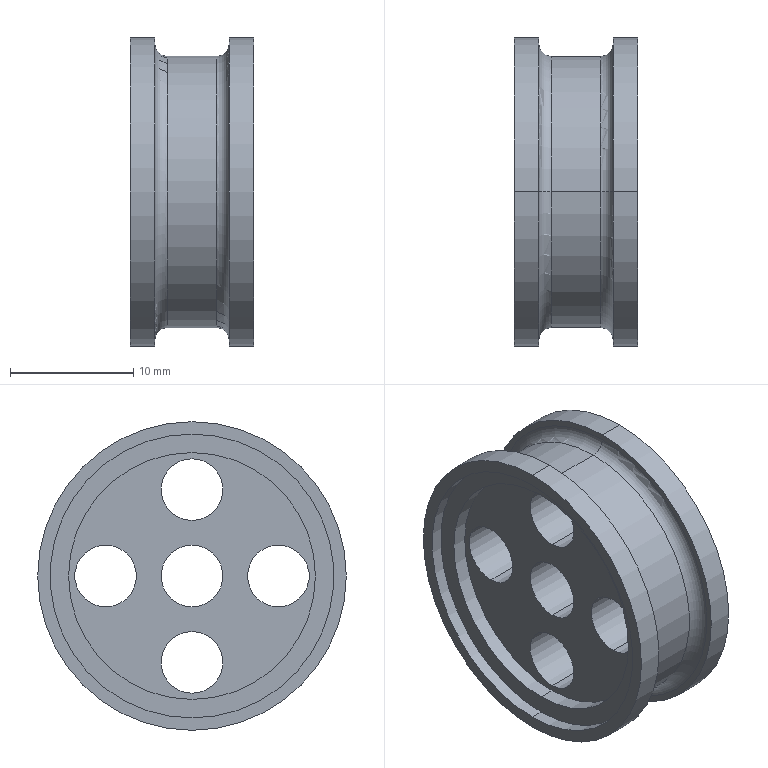Part | SolidWorks | features ICE 3, MirrorPattern 2, Revolution 1 | 1 solid | 36 faces | box 10 x 25 x 25 mm | volume 2118 mm3 | cylinder 24 | plane 8 | torus 4 | commonest cylinder face diameters 5 x10 20 x4 23 x4 25 x4 22 x2
STEP:
#1=CARTESIAN_POINT('',(-2.75,7.,-2.5));
#2=VERTEX_POINT('',#1);
#3=CARTESIAN_POINT('',(-2.75,7.,2.5));
#4=VERTEX_POINT('',#3);
#5=CARTESIAN_POINT('',(-2.75,7.,0.));
#6=DIRECTION('',(-1.,0.,0.));
#7=DIRECTION('',(0.,0.,1.));
#8=AXIS2_PLACEMENT_3D('',#5,#6,#7);
#9=CIRCLE('',#8,2.5);
#10=EDGE_CURVE('',#2,#4,#9,.T.);
#11=ORIENTED_EDGE('',*,*,#10,.T.);
#12=CARTESIAN_POINT('',(2.75,7.,2.5));
#13=VERTEX_POINT('',#12);
#14=CARTESIAN_POINT('',(-5.75,7.,2.5));
#15=DIRECTION('',(1.,0.,0.));
#16=VECTOR('',#15,1000.);
#17=LINE('',#14,#16);
#18=EDGE_CURVE('',#4,#13,#17,.T.);
#19=ORIENTED_EDGE('',*,*,#18,.T.);
#20=CARTESIAN_POINT('',(2.75,7.,-2.5));
#21=VERTEX_POINT('',#20);
#22=CARTESIAN_POINT('',(2.75,7.,0.));
#23=DIRECTION('',(1.,0.,0.));
#24=DIRECTION('',(0.,0.,-1.));
#25=AXIS2_PLACEMENT_3D('',#22,#23,#24);
#26=CIRCLE('',#25,2.5);
#27=EDGE_CURVE('',#13,#21,#26,.T.);
#28=ORIENTED_EDGE('',*,*,#27,.T.);
#29=CARTESIAN_POINT('',(-5.75,7.,-2.5));
#30=DIRECTION('',(1.,0.,0.));
#31=VECTOR('',#30,1000.);
#32=LINE('',#29,#31);
#33=EDGE_CURVE('',#2,#21,#32,.T.);
#34=ORIENTED_EDGE('',*,*,#33,.F.);
#35=EDGE_LOOP('',(#11,#19,#28,#34));
#36=FACE_OUTER_BOUND('',#35,.T.);
#37=CARTESIAN_POINT('',(-5.75,7.,0.));
#38=DIRECTION('',(1.,0.,0.));
#39=DIRECTION('',(0.,0.,-1.));
#40=AXIS2_PLACEMENT_3D('',#37,#38,#39);
#41=CYLINDRICAL_SURFACE('',#40,2.5);
#42=ADVANCED_FACE('',(#36),#41,.F.);
#43=CARTESIAN_POINT('',(-2.75,0.,4.5));
#44=VERTEX_POINT('',#43);
#45=CARTESIAN_POINT('',(-2.75,0.,9.5));
#46=VERTEX_POINT('',#45);
#47=CARTESIAN_POINT('',(-2.75,0.,7.));
#48=DIRECTION('',(-1.,0.,0.));
#49=DIRECTION('',(0.,0.,1.));
#50=AXIS2_PLACEMENT_3D('',#47,#48,#49);
#51=CIRCLE('',#50,2.5);
#52=EDGE_CURVE('',#44,#46,#51,.T.);
#53=ORIENTED_EDGE('',*,*,#52,.T.);
#54=CARTESIAN_POINT('',(2.75,0.,9.5));
#55=VERTEX_POINT('',#54);
#56=CARTESIAN_POINT('',(-5.75,0.,9.5));
#57=DIRECTION('',(1.,0.,0.));
#58=VECTOR('',#57,1000.);
#59=LINE('',#56,#58);
#60=EDGE_CURVE('',#46,#55,#59,.T.);
#61=ORIENTED_EDGE('',*,*,#60,.T.);
#62=CARTESIAN_POINT('',(2.75,0.,4.5));
#63=VERTEX_POINT('',#62);
#64=CARTESIAN_POINT('',(2.75,0.,7.));
#65=DIRECTION('',(1.,0.,0.));
#66=DIRECTION('',(0.,0.,-1.));
#67=AXIS2_PLACEMENT_3D('',#64,#65,#66);
#68=CIRCLE('',#67,2.5);
#69=EDGE_CURVE('',#55,#63,#68,.T.);
#70=ORIENTED_EDGE('',*,*,#69,.T.);
#71=CARTESIAN_POINT('',(-5.75,0.,4.5));
#72=DIRECTION('',(1.,0.,0.));
#73=VECTOR('',#72,1000.);
#74=LINE('',#71,#73);
#75=EDGE_CURVE('',#44,#63,#74,.T.);
#76=ORIENTED_EDGE('',*,*,#75,.F.);
#77=EDGE_LOOP('',(#53,#61,#70,#76));
#78=FACE_OUTER_BOUND('',#77,.T.);
#79=CARTESIAN_POINT('',(-5.75,0.,7.));
#80=DIRECTION('',(1.,0.,0.));
#81=DIRECTION('',(0.,0.,-1.));
#82=AXIS2_PLACEMENT_3D('',#79,#80,#81);
#83=CYLINDRICAL_SURFACE('',#82,2.5);
#84=ADVANCED_FACE('',(#78),#83,.F.);
#85=CARTESIAN_POINT('',(-2.75,-7.,-2.5));
#86=VERTEX_POINT('',#85);
#87=CARTESIAN_POINT('',(-2.75,-7.,2.5));
#88=VERTEX_POINT('',#87);
#89=CARTESIAN_POINT('',(-2.75,-7.,0.));
#90=DIRECTION('',(-1.,0.,0.));
#91=DIRECTION('',(0.,0.,1.));
#92=AXIS2_PLACEMENT_3D('',#89,#90,#91);
#93=CIRCLE('',#92,2.5);
#94=EDGE_CURVE('',#86,#88,#93,.T.);
#95=ORIENTED_EDGE('',*,*,#94,.T.);
#96=CARTESIAN_POINT('',(2.75,-7.,2.5));
#97=VERTEX_POINT('',#96);
#98=CARTESIAN_POINT('',(-5.75,-7.,2.5));
#99=DIRECTION('',(1.,0.,0.));
#100=VECTOR('',#99,1000.);
#101=LINE('',#98,#100);
#102=EDGE_CURVE('',#88,#97,#101,.T.);
#103=ORIENTED_EDGE('',*,*,#102,.T.);
#104=CARTESIAN_POINT('',(2.75,-7.,-2.5));
#105=VERTEX_POINT('',#104);
#106=CARTESIAN_POINT('',(2.75,-7.,0.));
#107=DIRECTION('',(1.,0.,0.));
#108=DIRECTION('',(0.,0.,-1.));
#109=AXIS2_PLACEMENT_3D('',#106,#107,#108);
#110=CIRCLE('',#109,2.5);
#111=EDGE_CURVE('',#97,#105,#110,.T.);
#112=ORIENTED_EDGE('',*,*,#111,.T.);
#113=CARTESIAN_POINT('',(-5.75,-7.,-2.5));
#114=DIRECTION('',(1.,0.,0.));
#115=VECTOR('',#114,1000.);
#116=LINE('',#113,#115);
#117=EDGE_CURVE('',#86,#105,#116,.T.);
#118=ORIENTED_EDGE('',*,*,#117,.F.);
#119=EDGE_LOOP('',(#95,#103,#112,#118));
#120=FACE_OUTER_BOUND('',#119,.T.);
#121=CARTESIAN_POINT('',(-5.75,-7.,0.));
#122=DIRECTION('',(1.,0.,0.));
#123=DIRECTION('',(0.,0.,-1.));
#124=AXIS2_PLACEMENT_3D('',#121,#122,#123);
#125=CYLINDRICAL_SURFACE('',#124,2.5);
#126=ADVANCED_FACE('',(#120),#125,.F.);
#127=CARTESIAN_POINT('',(-2.75,0.,-9.5));
#128=VERTEX_POINT('',#127);
#129=CARTESIAN_POINT('',(-2.75,0.,-4.5));
#130=VERTEX_POINT('',#129);
#131=CARTESIAN_POINT('',(-2.75,0.,-7.));
#132=DIRECTION('',(-1.,0.,0.));
#133=DIRECTION('',(0.,0.,1.));
#134=AXIS2_PLACEMENT_3D('',#131,#132,#133);
#135=CIRCLE('',#134,2.5);
#136=EDGE_CURVE('',#128,#130,#135,.T.);
#137=ORIENTED_EDGE('',*,*,#136,.T.);
#138=CARTESIAN_POINT('',(2.75,0.,-4.5));
#139=VERTEX_POINT('',#138);
#140=CARTESIAN_POINT('',(-5.75,0.,-4.5));
#141=DIRECTION('',(1.,0.,0.));
#142=VECTOR('',#141,1000.);
#143=LINE('',#140,#142);
#144=EDGE_CURVE('',#130,#139,#143,.T.);
#145=ORIENTED_EDGE('',*,*,#144,.T.);
#146=CARTESIAN_POINT('',(2.75,0.,-9.5));
#147=VERTEX_POINT('',#146);
#148=CARTESIAN_POINT('',(2.75,0.,-7.));
#149=DIRECTION('',(1.,0.,0.));
#150=DIRECTION('',(0.,0.,-1.));
#151=AXIS2_PLACEMENT_3D('',#148,#149,#150);
#152=CIRCLE('',#151,2.5);
#153=EDGE_CURVE('',#139,#147,#152,.T.);
#154=ORIENTED_EDGE('',*,*,#153,.T.);
#155=CARTESIAN_POINT('',(-5.75,0.,-9.5));
#156=DIRECTION('',(1.,0.,0.));
#157=VECTOR('',#156,1000.);
#158=LINE('',#155,#157);
#159=EDGE_CURVE('',#128,#147,#158,.T.);
#160=ORIENTED_EDGE('',*,*,#159,.F.);
#161=EDGE_LOOP('',(#137,#145,#154,#160));
#162=FACE_OUTER_BOUND('',#161,.T.);
#163=CARTESIAN_POINT('',(-5.75,0.,-7.));
#164=DIRECTION('',(1.,0.,0.));
#165=DIRECTION('',(0.,0.,-1.));
#166=AXIS2_PLACEMENT_3D('',#163,#164,#165);
#167=CYLINDRICAL_SURFACE('',#166,2.5);
#168=ADVANCED_FACE('',(#162),#167,.F.);
#169=CARTESIAN_POINT('',(-2.75,0.,-2.5));
#170=VERTEX_POINT('',#169);
#171=CARTESIAN_POINT('',(-2.75,0.,2.5));
#172=VERTEX_POINT('',#171);
#173=CARTESIAN_POINT('',(-2.75,0.,0.));
#174=DIRECTION('',(-1.,0.,0.));
#175=DIRECTION('',(0.,0.,1.));
#176=AXIS2_PLACEMENT_3D('',#173,#174,#175);
#177=CIRCLE('',#176,2.5);
#178=EDGE_CURVE('',#170,#172,#177,.T.);
#179=ORIENTED_EDGE('',*,*,#178,.T.);
#180=CARTESIAN_POINT('',(2.75,0.,2.5));
#181=VERTEX_POINT('',#180);
#182=CARTESIAN_POINT('',(-5.75,0.,2.5));
#183=DIRECTION('',(1.,0.,0.));
#184=VECTOR('',#183,1000.);
#185=LINE('',#182,#184);
#186=EDGE_CURVE('',#172,#181,#185,.T.);
#187=ORIENTED_EDGE('',*,*,#186,.T.);
#188=CARTESIAN_POINT('',(2.75,0.,-2.5));
#189=VERTEX_POINT('',#188);
#190=CARTESIAN_POINT('',(2.75,0.,0.));
#191=DIRECTION('',(1.,0.,0.));
#192=DIRECTION('',(0.,0.,-1.));
#193=AXIS2_PLACEMENT_3D('',#190,#191,#192);
#194=CIRCLE('',#193,2.5);
#195=EDGE_CURVE('',#181,#189,#194,.T.);
#196=ORIENTED_EDGE('',*,*,#195,.T.);
#197=CARTESIAN_POINT('',(-5.75,0.,-2.5));
#198=DIRECTION('',(1.,0.,0.));
#199=VECTOR('',#198,1000.);
#200=LINE('',#197,#199);
#201=EDGE_CURVE('',#170,#189,#200,.T.);
#202=ORIENTED_EDGE('',*,*,#201,.F.);
#203=EDGE_LOOP('',(#179,#187,#196,#202));
#204=FACE_OUTER_BOUND('',#203,.T.);
#205=CARTESIAN_POINT('',(-5.75,0.,0.));
#206=DIRECTION('',(1.,0.,0.));
#207=DIRECTION('',(0.,0.,-1.));
#208=AXIS2_PLACEMENT_3D('',#205,#206,#207);
#209=CYLINDRICAL_SURFACE('',#208,2.5);
#210=ADVANCED_FACE('',(#204),#209,.F.);
#211=CARTESIAN_POINT('',(-2.75,0.,10.));
#212=VERTEX_POINT('',#211);
#213=CARTESIAN_POINT('',(-2.75,0.,-10.));
#214=VERTEX_POINT('',#213);
#215=CARTESIAN_POINT('',(-2.75,0.,0.));
#216=DIRECTION('',(1.,0.,0.));
#217=DIRECTION('',(0.,0.,-1.));
#218=AXIS2_PLACEMENT_3D('',#215,#216,#217);
#219=CIRCLE('',#218,10.);
#220=EDGE_CURVE('',#212,#214,#219,.T.);
#221=ORIENTED_EDGE('',*,*,#220,.T.);
#222=CARTESIAN_POINT('',(-4.,0.,-10.));
#223=VERTEX_POINT('',#222);
#224=CARTESIAN_POINT('',(-2.75,0.,-10.));
#225=DIRECTION('',(-1.,0.,0.));
#226=VECTOR('',#225,1000.);
#227=LINE('',#224,#226);
#228=EDGE_CURVE('',#214,#223,#227,.T.);
#229=ORIENTED_EDGE('',*,*,#228,.T.);
#230=CARTESIAN_POINT('',(-4.,0.,10.));
#231=VERTEX_POINT('',#230);
#232=CARTESIAN_POINT('',(-4.,0.,0.));
#233=DIRECTION('',(1.,0.,0.));
#234=DIRECTION('',(0.,0.,-1.));
#235=AXIS2_PLACEMENT_3D('',#232,#233,#234);
#236=CIRCLE('',#235,10.);
#237=EDGE_CURVE('',#231,#223,#236,.T.);
#238=ORIENTED_EDGE('',*,*,#237,.F.);
#239=CARTESIAN_POINT('',(-2.75,0.,10.));
#240=DIRECTION('',(-1.,0.,0.));
#241=VECTOR('',#240,1000.);
#242=LINE('',#239,#241);
#243=EDGE_CURVE('',#212,#231,#242,.T.);
#244=ORIENTED_EDGE('',*,*,#243,.F.);
#245=EDGE_LOOP('',(#221,#229,#238,#244));
#246=FACE_OUTER_BOUND('',#245,.T.);
#247=CARTESIAN_POINT('',(-2.75,0.,0.));
#248=DIRECTION('',(-1.,0.,0.));
#249=DIRECTION('',(0.,0.,1.));
#250=AXIS2_PLACEMENT_3D('',#247,#248,#249);
#251=CYLINDRICAL_SURFACE('',#250,10.);
#252=ADVANCED_FACE('',(#246),#251,.F.);
#253=CARTESIAN_POINT('',(-4.,0.,11.5));
#254=VERTEX_POINT('',#253);
#255=CARTESIAN_POINT('',(-4.,0.,-11.5));
#256=VERTEX_POINT('',#255);
#257=CARTESIAN_POINT('',(-4.,0.,0.));
#258=DIRECTION('',(1.,0.,0.));
#259=DIRECTION('',(0.,0.,-1.));
#260=AXIS2_PLACEMENT_3D('',#257,#258,#259);
#261=CIRCLE('',#260,11.5);
#262=EDGE_CURVE('',#254,#256,#261,.T.);
#263=ORIENTED_EDGE('',*,*,#262,.T.);
#264=CARTESIAN_POINT('',(-5.,0.,-11.5));
#265=VERTEX_POINT('',#264);
#266=CARTESIAN_POINT('',(-4.,0.,-11.5));
#267=DIRECTION('',(-1.,0.,0.));
#268=VECTOR('',#267,1000.);
#269=LINE('',#266,#268);
#270=EDGE_CURVE('',#256,#265,#269,.T.);
#271=ORIENTED_EDGE('',*,*,#270,.T.);
#272=CARTESIAN_POINT('',(-5.,0.,11.5));
#273=VERTEX_POINT('',#272);
#274=CARTESIAN_POINT('',(-5.,0.,0.));
#275=DIRECTION('',(1.,0.,0.));
#276=DIRECTION('',(0.,0.,-1.));
#277=AXIS2_PLACEMENT_3D('',#274,#275,#276);
#278=CIRCLE('',#277,11.5);
#279=EDGE_CURVE('',#273,#265,#278,.T.);
#280=ORIENTED_EDGE('',*,*,#279,.F.);
#281=CARTESIAN_POINT('',(-4.,0.,11.5));
#282=DIRECTION('',(-1.,0.,0.));
#283=VECTOR('',#282,1000.);
#284=LINE('',#281,#283);
#285=EDGE_CURVE('',#254,#273,#284,.T.);
#286=ORIENTED_EDGE('',*,*,#285,.F.);
#287=EDGE_LOOP('',(#263,#271,#280,#286));
#288=FACE_OUTER_BOUND('',#287,.T.);
#289=CARTESIAN_POINT('',(-4.,0.,0.));
#290=DIRECTION('',(-1.,0.,0.));
#291=DIRECTION('',(0.,0.,1.));
#292=AXIS2_PLACEMENT_3D('',#289,#290,#291);
#293=CYLINDRICAL_SURFACE('',#292,11.5);
#294=ADVANCED_FACE('',(#288),#293,.F.);
#295=CARTESIAN_POINT('',(2.75,0.,10.));
#296=VERTEX_POINT('',#295);
#297=CARTESIAN_POINT('',(2.75,0.,-10.));
#298=VERTEX_POINT('',#297);
#299=CARTESIAN_POINT('',(2.75,0.,0.));
#300=DIRECTION('',(1.,0.,0.));
#301=DIRECTION('',(0.,0.,-1.));
#302=AXIS2_PLACEMENT_3D('',#299,#300,#301);
#303=CIRCLE('',#302,10.);
#304=EDGE_CURVE('',#296,#298,#303,.T.);
#305=ORIENTED_EDGE('',*,*,#304,.F.);
#306=CARTESIAN_POINT('',(4.,0.,10.));
#307=VERTEX_POINT('',#306);
#308=CARTESIAN_POINT('',(2.75,0.,10.));
#309=DIRECTION('',(1.,0.,0.));
#310=VECTOR('',#309,1000.);
#311=LINE('',#308,#310);
#312=EDGE_CURVE('',#296,#307,#311,.T.);
#313=ORIENTED_EDGE('',*,*,#312,.T.);
#314=CARTESIAN_POINT('',(4.,0.,-10.));
#315=VERTEX_POINT('',#314);
#316=CARTESIAN_POINT('',(4.,0.,0.));
#317=DIRECTION('',(1.,0.,0.));
#318=DIRECTION('',(0.,0.,-1.));
#319=AXIS2_PLACEMENT_3D('',#316,#317,#318);
#320=CIRCLE('',#319,10.);
#321=EDGE_CURVE('',#307,#315,#320,.T.);
#322=ORIENTED_EDGE('',*,*,#321,.T.);
#323=CARTESIAN_POINT('',(2.75,0.,-10.));
#324=DIRECTION('',(1.,0.,0.));
#325=VECTOR('',#324,1000.);
#326=LINE('',#323,#325);
#327=EDGE_CURVE('',#298,#315,#326,.T.);
#328=ORIENTED_EDGE('',*,*,#327,.F.);
#329=EDGE_LOOP('',(#305,#313,#322,#328));
#330=FACE_OUTER_BOUND('',#329,.T.);
#331=CARTESIAN_POINT('',(2.75,0.,0.));
#332=DIRECTION('',(1.,0.,0.));
#333=DIRECTION('',(0.,0.,-1.));
#334=AXIS2_PLACEMENT_3D('',#331,#332,#333);
#335=CYLINDRICAL_SURFACE('',#334,10.);
#336=ADVANCED_FACE('',(#330),#335,.F.);
#337=CARTESIAN_POINT('',(4.,0.,11.5));
#338=VERTEX_POINT('',#337);
#339=CARTESIAN_POINT('',(4.,0.,-11.5));
#340=VERTEX_POINT('',#339);
#341=CARTESIAN_POINT('',(4.,0.,0.));
#342=DIRECTION('',(1.,0.,0.));
#343=DIRECTION('',(0.,0.,-1.));
#344=AXIS2_PLACEMENT_3D('',#341,#342,#343);
#345=CIRCLE('',#344,11.5);
#346=EDGE_CURVE('',#338,#340,#345,.T.);
#347=ORIENTED_EDGE('',*,*,#346,.F.);
#348=CARTESIAN_POINT('',(5.,0.,11.5));
#349=VERTEX_POINT('',#348);
#350=CARTESIAN_POINT('',(4.,0.,11.5));
#351=DIRECTION('',(1.,0.,0.));
#352=VECTOR('',#351,1000.);
#353=LINE('',#350,#352);
#354=EDGE_CURVE('',#338,#349,#353,.T.);
#355=ORIENTED_EDGE('',*,*,#354,.T.);
#356=CARTESIAN_POINT('',(5.,0.,-11.5));
#357=VERTEX_POINT('',#356);
#358=CARTESIAN_POINT('',(5.,0.,0.));
#359=DIRECTION('',(1.,0.,0.));
#360=DIRECTION('',(0.,0.,-1.));
#361=AXIS2_PLACEMENT_3D('',#358,#359,#360);
#362=CIRCLE('',#361,11.5);
#363=EDGE_CURVE('',#349,#357,#362,.T.);
#364=ORIENTED_EDGE('',*,*,#363,.T.);
#365=CARTESIAN_POINT('',(4.,0.,-11.5));
#366=DIRECTION('',(1.,0.,0.));
#367=VECTOR('',#366,1000.);
#368=LINE('',#365,#367);
#369=EDGE_CURVE('',#340,#357,#368,.T.);
#370=ORIENTED_EDGE('',*,*,#369,.F.);
#371=EDGE_LOOP('',(#347,#355,#364,#370));
#372=FACE_OUTER_BOUND('',#371,.T.);
#373=CARTESIAN_POINT('',(4.,0.,0.));
#374=DIRECTION('',(1.,0.,0.));
#375=DIRECTION('',(0.,0.,-1.));
#376=AXIS2_PLACEMENT_3D('',#373,#374,#375);
#377=CYLINDRICAL_SURFACE('',#376,11.5);
#378=ADVANCED_FACE('',(#372),#377,.F.);
#379=CARTESIAN_POINT('',(-5.,0.,-12.5));
#380=VERTEX_POINT('',#379);
#381=CARTESIAN_POINT('',(-5.,0.,12.5));
#382=VERTEX_POINT('',#381);
#383=CARTESIAN_POINT('',(-5.,0.,0.));
#384=DIRECTION('',(-1.,0.,0.));
#385=DIRECTION('',(0.,0.,1.));
#386=AXIS2_PLACEMENT_3D('',#383,#384,#385);
#387=CIRCLE('',#386,12.5);
#388=EDGE_CURVE('',#380,#382,#387,.T.);
#389=ORIENTED_EDGE('',*,*,#388,.F.);
#390=CARTESIAN_POINT('',(-3.,0.,-12.5));
#391=VERTEX_POINT('',#390);
#392=CARTESIAN_POINT('',(0.,0.,-12.5));
#393=DIRECTION('',(1.,0.,0.));
#394=VECTOR('',#393,1000.);
#395=LINE('',#392,#394);
#396=EDGE_CURVE('',#380,#391,#395,.T.);
#397=ORIENTED_EDGE('',*,*,#396,.T.);
#398=CARTESIAN_POINT('',(-3.,0.,12.5));
#399=VERTEX_POINT('',#398);
#400=CARTESIAN_POINT('',(-3.,0.,0.));
#401=DIRECTION('',(-1.,0.,0.));
#402=DIRECTION('',(0.,0.,1.));
#403=AXIS2_PLACEMENT_3D('',#400,#401,#402);
#404=CIRCLE('',#403,12.5);
#405=EDGE_CURVE('',#391,#399,#404,.T.);
#406=ORIENTED_EDGE('',*,*,#405,.T.);
#407=CARTESIAN_POINT('',(0.,0.,12.5));
#408=DIRECTION('',(1.,0.,0.));
#409=VECTOR('',#408,1000.);
#410=LINE('',#407,#409);
#411=EDGE_CURVE('',#382,#399,#410,.T.);
#412=ORIENTED_EDGE('',*,*,#411,.F.);
#413=EDGE_LOOP('',(#389,#397,#406,#412));
#414=FACE_OUTER_BOUND('',#413,.T.);
#415=CARTESIAN_POINT('',(0.,0.,0.));
#416=DIRECTION('',(1.,0.,0.));
#417=DIRECTION('',(0.,0.,1.));
#418=AXIS2_PLACEMENT_3D('',#415,#416,#417);
#419=CYLINDRICAL_SURFACE('',#418,12.5);
#420=ADVANCED_FACE('',(#414),#419,.T.);
#421=CARTESIAN_POINT('',(-2.,0.,11.));
#422=VERTEX_POINT('',#421);
#423=CARTESIAN_POINT('',(-2.,0.,-11.));
#424=VERTEX_POINT('',#423);
#425=CARTESIAN_POINT('',(-2.,0.,0.));
#426=DIRECTION('',(-1.,0.,0.));
#427=DIRECTION('',(0.,0.,1.));
#428=AXIS2_PLACEMENT_3D('',#425,#426,#427);
#429=CIRCLE('',#428,11.);
#430=EDGE_CURVE('',#422,#424,#429,.T.);
#431=ORIENTED_EDGE('',*,*,#430,.T.);
#432=CARTESIAN_POINT('',(-3.,0.,-12.));
#433=VERTEX_POINT('',#432);
#434=CARTESIAN_POINT('',(-2.,0.,-12.));
#435=DIRECTION('',(0.,-1.,0.));
#436=DIRECTION('',(0.,0.,-1.));
#437=AXIS2_PLACEMENT_3D('',#434,#435,#436);
#438=CIRCLE('',#437,1.);
#439=EDGE_CURVE('',#424,#433,#438,.T.);
#440=ORIENTED_EDGE('',*,*,#439,.T.);
#441=CARTESIAN_POINT('',(-3.,0.,12.));
#442=VERTEX_POINT('',#441);
#443=CARTESIAN_POINT('',(-3.,0.,0.));
#444=DIRECTION('',(-1.,0.,0.));
#445=DIRECTION('',(0.,0.,1.));
#446=AXIS2_PLACEMENT_3D('',#443,#444,#445);
#447=CIRCLE('',#446,12.);
#448=EDGE_CURVE('',#442,#433,#447,.T.);
#449=ORIENTED_EDGE('',*,*,#448,.F.);
#450=CARTESIAN_POINT('',(-2.,0.,12.));
#451=DIRECTION('',(0.,1.,0.));
#452=DIRECTION('',(0.,0.,1.));
#453=AXIS2_PLACEMENT_3D('',#450,#451,#452);
#454=CIRCLE('',#453,1.);
#455=EDGE_CURVE('',#422,#442,#454,.T.);
#456=ORIENTED_EDGE('',*,*,#455,.F.);
#457=EDGE_LOOP('',(#431,#440,#449,#456));
#458=FACE_OUTER_BOUND('',#457,.T.);
#459=CARTESIAN_POINT('',(-2.,0.,0.));
#460=DIRECTION('',(1.,0.,0.));
#461=DIRECTION('',(0.,0.,1.));
#462=AXIS2_PLACEMENT_3D('',#459,#460,#461);
#463=TOROIDAL_SURFACE('',#462,12.,1.);
#464=ADVANCED_FACE('',(#458),#463,.F.);
#465=CARTESIAN_POINT('',(5.,0.,12.5));
#466=VERTEX_POINT('',#465);
#467=CARTESIAN_POINT('',(5.,0.,-12.5));
#468=VERTEX_POINT('',#467);
#469=CARTESIAN_POINT('',(5.,0.,0.));
#470=DIRECTION('',(-1.,0.,0.));
#471=DIRECTION('',(0.,0.,1.));
#472=AXIS2_PLACEMENT_3D('',#469,#470,#471);
#473=CIRCLE('',#472,12.5);
#474=EDGE_CURVE('',#466,#468,#473,.T.);
#475=ORIENTED_EDGE('',*,*,#474,.T.);
#476=CARTESIAN_POINT('',(3.,0.,-12.5));
#477=VERTEX_POINT('',#476);
#478=CARTESIAN_POINT('',(0.,0.,-12.5));
#479=DIRECTION('',(-1.,0.,0.));
#480=VECTOR('',#479,1000.);
#481=LINE('',#478,#480);
#482=EDGE_CURVE('',#468,#477,#481,.T.);
#483=ORIENTED_EDGE('',*,*,#482,.T.);
#484=CARTESIAN_POINT('',(3.,0.,12.5));
#485=VERTEX_POINT('',#484);
#486=CARTESIAN_POINT('',(3.,0.,0.));
#487=DIRECTION('',(-1.,0.,0.));
#488=DIRECTION('',(0.,0.,1.));
#489=AXIS2_PLACEMENT_3D('',#486,#487,#488);
#490=CIRCLE('',#489,12.5);
#491=EDGE_CURVE('',#485,#477,#490,.T.);
#492=ORIENTED_EDGE('',*,*,#491,.F.);
#493=CARTESIAN_POINT('',(0.,0.,12.5));
#494=DIRECTION('',(-1.,0.,0.));
#495=VECTOR('',#494,1000.);
#496=LINE('',#493,#495);
#497=EDGE_CURVE('',#466,#485,#496,.T.);
#498=ORIENTED_EDGE('',*,*,#497,.F.);
#499=EDGE_LOOP('',(#475,#483,#492,#498));
#500=FACE_OUTER_BOUND('',#499,.T.);
#501=CARTESIAN_POINT('',(0.,0.,0.));
#502=DIRECTION('',(-1.,0.,0.));
#503=DIRECTION('',(0.,0.,1.));
#504=AXIS2_PLACEMENT_3D('',#501,#502,#503);
#505=CYLINDRICAL_SURFACE('',#504,12.5);
#506=ADVANCED_FACE('',(#500),#505,.T.);
#507=CARTESIAN_POINT('',(2.,0.,-11.));
#508=VERTEX_POINT('',#507);
#509=CARTESIAN_POINT('',(2.,0.,11.));
#510=VERTEX_POINT('',#509);
#511=CARTESIAN_POINT('',(2.,0.,0.));
#512=DIRECTION('',(-1.,0.,0.));
#513=DIRECTION('',(0.,0.,1.));
#514=AXIS2_PLACEMENT_3D('',#511,#512,#513);
#515=CIRCLE('',#514,11.);
#516=EDGE_CURVE('',#508,#510,#515,.T.);
#517=ORIENTED_EDGE('',*,*,#516,.F.);
#518=CARTESIAN_POINT('',(3.,0.,-12.));
#519=VERTEX_POINT('',#518);
#520=CARTESIAN_POINT('',(2.,0.,-12.));
#521=DIRECTION('',(0.,1.,0.));
#522=DIRECTION('',(0.,0.,1.));
#523=AXIS2_PLACEMENT_3D('',#520,#521,#522);
#524=CIRCLE('',#523,1.);
#525=EDGE_CURVE('',#508,#519,#524,.T.);
#526=ORIENTED_EDGE('',*,*,#525,.T.);
#527=CARTESIAN_POINT('',(3.,0.,12.));
#528=VERTEX_POINT('',#527);
#529=CARTESIAN_POINT('',(3.,0.,0.));
#530=DIRECTION('',(-1.,0.,0.));
#531=DIRECTION('',(0.,0.,1.));
#532=AXIS2_PLACEMENT_3D('',#529,#530,#531);
#533=CIRCLE('',#532,12.);
#534=EDGE_CURVE('',#519,#528,#533,.T.);
#535=ORIENTED_EDGE('',*,*,#534,.T.);
#536=CARTESIAN_POINT('',(2.,0.,12.));
#537=DIRECTION('',(0.,-1.,0.));
#538=DIRECTION('',(0.,0.,-1.));
#539=AXIS2_PLACEMENT_3D('',#536,#537,#538);
#540=CIRCLE('',#539,1.);
#541=EDGE_CURVE('',#510,#528,#540,.T.);
#542=ORIENTED_EDGE('',*,*,#541,.F.);
#543=EDGE_LOOP('',(#517,#526,#535,#542));
#544=FACE_OUTER_BOUND('',#543,.T.);
#545=CARTESIAN_POINT('',(2.,0.,0.));
#546=DIRECTION('',(-1.,0.,0.));
#547=DIRECTION('',(0.,0.,1.));
#548=AXIS2_PLACEMENT_3D('',#545,#546,#547);
#549=TOROIDAL_SURFACE('',#548,12.,1.);
#550=ADVANCED_FACE('',(#544),#549,.F.);
#551=CARTESIAN_POINT('',(2.,0.,0.));
#552=DIRECTION('',(-1.,0.,0.));
#553=DIRECTION('',(0.,0.,1.));
#554=AXIS2_PLACEMENT_3D('',#551,#552,#553);
#555=CIRCLE('',#554,11.);
#556=EDGE_CURVE('',#510,#508,#555,.T.);
#557=ORIENTED_EDGE('',*,*,#556,.T.);
#558=CARTESIAN_POINT('',(0.,0.,-11.));
#559=DIRECTION('',(-1.,0.,0.));
#560=VECTOR('',#559,1000.);
#561=LINE('',#558,#560);
#562=EDGE_CURVE('',#508,#424,#561,.T.);
#563=ORIENTED_EDGE('',*,*,#562,.T.);
#564=ORIENTED_EDGE('',*,*,#430,.F.);
#565=CARTESIAN_POINT('',(0.,0.,11.));
#566=DIRECTION('',(-1.,0.,0.));
#567=VECTOR('',#566,1000.);
#568=LINE('',#565,#567);
#569=EDGE_CURVE('',#510,#422,#568,.T.);
#570=ORIENTED_EDGE('',*,*,#569,.F.);
#571=EDGE_LOOP('',(#557,#563,#564,#570));
#572=FACE_OUTER_BOUND('',#571,.T.);
#573=CARTESIAN_POINT('',(0.,0.,0.));
#574=DIRECTION('',(-1.,0.,0.));
#575=DIRECTION('',(0.,0.,1.));
#576=AXIS2_PLACEMENT_3D('',#573,#574,#575);
#577=CYLINDRICAL_SURFACE('',#576,11.);
#578=ADVANCED_FACE('',(#572),#577,.T.);
#579=ORIENTED_EDGE('',*,*,#562,.F.);
#580=ORIENTED_EDGE('',*,*,#516,.T.);
#581=ORIENTED_EDGE('',*,*,#569,.T.);
#582=CARTESIAN_POINT('',(-2.,0.,0.));
#583=DIRECTION('',(-1.,0.,0.));
#584=DIRECTION('',(0.,0.,1.));
#585=AXIS2_PLACEMENT_3D('',#582,#583,#584);
#586=CIRCLE('',#585,11.);
#587=EDGE_CURVE('',#424,#422,#586,.T.);
#588=ORIENTED_EDGE('',*,*,#587,.F.);
#589=EDGE_LOOP('',(#579,#580,#581,#588));
#590=FACE_OUTER_BOUND('',#589,.T.);
#591=CARTESIAN_POINT('',(0.,0.,0.));
#592=DIRECTION('',(-1.,0.,0.));
#593=DIRECTION('',(0.,0.,1.));
#594=AXIS2_PLACEMENT_3D('',#591,#592,#593);
#595=CYLINDRICAL_SURFACE('',#594,11.);
#596=ADVANCED_FACE('',(#590),#595,.T.);
#597=ORIENTED_EDGE('',*,*,#525,.F.);
#598=ORIENTED_EDGE('',*,*,#556,.F.);
#599=ORIENTED_EDGE('',*,*,#541,.T.);
#600=CARTESIAN_POINT('',(3.,0.,0.));
#601=DIRECTION('',(-1.,0.,0.));
#602=DIRECTION('',(0.,0.,1.));
#603=AXIS2_PLACEMENT_3D('',#600,#601,#602);
#604=CIRCLE('',#603,12.);
#605=EDGE_CURVE('',#528,#519,#604,.T.);
#606=ORIENTED_EDGE('',*,*,#605,.T.);
#607=EDGE_LOOP('',(#597,#598,#599,#606));
#608=FACE_OUTER_BOUND('',#607,.T.);
#609=CARTESIAN_POINT('',(2.,0.,0.));
#610=DIRECTION('',(-1.,0.,0.));
#611=DIRECTION('',(0.,0.,1.));
#612=AXIS2_PLACEMENT_3D('',#609,#610,#611);
#613=TOROIDAL_SURFACE('',#612,12.,1.);
#614=ADVANCED_FACE('',(#608),#613,.F.);
#615=ORIENTED_EDGE('',*,*,#605,.F.);
#616=ORIENTED_EDGE('',*,*,#534,.F.);
#617=EDGE_LOOP('',(#615,#616));
#618=FACE_BOUND('',#617,.T.);
#619=ORIENTED_EDGE('',*,*,#491,.T.);
#620=CARTESIAN_POINT('',(3.,0.,0.));
#621=DIRECTION('',(-1.,0.,0.));
#622=DIRECTION('',(0.,0.,1.));
#623=AXIS2_PLACEMENT_3D('',#620,#621,#622);
#624=CIRCLE('',#623,12.5);
#625=EDGE_CURVE('',#477,#485,#624,.T.);
#626=ORIENTED_EDGE('',*,*,#625,.T.);
#627=EDGE_LOOP('',(#619,#626));
#628=FACE_OUTER_BOUND('',#627,.T.);
#629=CARTESIAN_POINT('',(3.,12.5,0.));
#630=DIRECTION('',(1.,0.,0.));
#631=DIRECTION('',(0.,0.,-1.));
#632=AXIS2_PLACEMENT_3D('',#629,#630,#631);
#633=PLANE('',#632);
#634=ADVANCED_FACE('',(#618,#628),#633,.F.);
#635=ORIENTED_EDGE('',*,*,#482,.F.);
#636=CARTESIAN_POINT('',(5.,0.,0.));
#637=DIRECTION('',(-1.,0.,0.));
#638=DIRECTION('',(0.,0.,1.));
#639=AXIS2_PLACEMENT_3D('',#636,#637,#638);
#640=CIRCLE('',#639,12.5);
#641=EDGE_CURVE('',#468,#466,#640,.T.);
#642=ORIENTED_EDGE('',*,*,#641,.T.);
#643=ORIENTED_EDGE('',*,*,#497,.T.);
#644=ORIENTED_EDGE('',*,*,#625,.F.);
#645=EDGE_LOOP('',(#635,#642,#643,#644));
#646=FACE_OUTER_BOUND('',#645,.T.);
#647=CARTESIAN_POINT('',(0.,0.,0.));
#648=DIRECTION('',(-1.,0.,0.));
#649=DIRECTION('',(0.,0.,1.));
#650=AXIS2_PLACEMENT_3D('',#647,#648,#649);
#651=CYLINDRICAL_SURFACE('',#650,12.5);
#652=ADVANCED_FACE('',(#646),#651,.T.);
#653=CARTESIAN_POINT('',(5.,0.,0.));
#654=DIRECTION('',(1.,0.,0.));
#655=DIRECTION('',(0.,0.,-1.));
#656=AXIS2_PLACEMENT_3D('',#653,#654,#655);
#657=CIRCLE('',#656,11.5);
#658=EDGE_CURVE('',#357,#349,#657,.T.);
#659=ORIENTED_EDGE('',*,*,#658,.F.);
#660=ORIENTED_EDGE('',*,*,#363,.F.);
#661=EDGE_LOOP('',(#659,#660));
#662=FACE_BOUND('',#661,.T.);
#663=ORIENTED_EDGE('',*,*,#474,.F.);
#664=ORIENTED_EDGE('',*,*,#641,.F.);
#665=EDGE_LOOP('',(#663,#664));
#666=FACE_OUTER_BOUND('',#665,.T.);
#667=CARTESIAN_POINT('',(5.,0.,0.));
#668=DIRECTION('',(-1.,0.,0.));
#669=DIRECTION('',(0.,0.,1.));
#670=AXIS2_PLACEMENT_3D('',#667,#668,#669);
#671=PLANE('',#670);
#672=ADVANCED_FACE('',(#662,#666),#671,.F.);
#673=ORIENTED_EDGE('',*,*,#439,.F.);
#674=ORIENTED_EDGE('',*,*,#587,.T.);
#675=ORIENTED_EDGE('',*,*,#455,.T.);
#676=CARTESIAN_POINT('',(-3.,0.,0.));
#677=DIRECTION('',(-1.,0.,0.));
#678=DIRECTION('',(0.,0.,1.));
#679=AXIS2_PLACEMENT_3D('',#676,#677,#678);
#680=CIRCLE('',#679,12.);
#681=EDGE_CURVE('',#433,#442,#680,.T.);
#682=ORIENTED_EDGE('',*,*,#681,.F.);
#683=EDGE_LOOP('',(#673,#674,#675,#682));
#684=FACE_OUTER_BOUND('',#683,.T.);
#685=CARTESIAN_POINT('',(-2.,0.,0.));
#686=DIRECTION('',(1.,0.,0.));
#687=DIRECTION('',(0.,0.,1.));
#688=AXIS2_PLACEMENT_3D('',#685,#686,#687);
#689=TOROIDAL_SURFACE('',#688,12.,1.);
#690=ADVANCED_FACE('',(#684),#689,.F.);
#691=ORIENTED_EDGE('',*,*,#448,.T.);
#692=ORIENTED_EDGE('',*,*,#681,.T.);
#693=EDGE_LOOP('',(#691,#692));
#694=FACE_BOUND('',#693,.T.);
#695=CARTESIAN_POINT('',(-3.,0.,0.));
#696=DIRECTION('',(-1.,0.,0.));
#697=DIRECTION('',(0.,0.,1.));
#698=AXIS2_PLACEMENT_3D('',#695,#696,#697);
#699=CIRCLE('',#698,12.5);
#700=EDGE_CURVE('',#399,#391,#699,.T.);
#701=ORIENTED_EDGE('',*,*,#700,.F.);
#702=ORIENTED_EDGE('',*,*,#405,.F.);
#703=EDGE_LOOP('',(#701,#702));
#704=FACE_OUTER_BOUND('',#703,.T.);
#705=CARTESIAN_POINT('',(-3.,12.5,0.));
#706=DIRECTION('',(-1.,0.,0.));
#707=DIRECTION('',(0.,0.,-1.));
#708=AXIS2_PLACEMENT_3D('',#705,#706,#707);
#709=PLANE('',#708);
#710=ADVANCED_FACE('',(#694,#704),#709,.F.);
#711=ORIENTED_EDGE('',*,*,#396,.F.);
#712=CARTESIAN_POINT('',(-5.,0.,0.));
#713=DIRECTION('',(-1.,0.,0.));
#714=DIRECTION('',(0.,0.,1.));
#715=AXIS2_PLACEMENT_3D('',#712,#713,#714);
#716=CIRCLE('',#715,12.5);
#717=EDGE_CURVE('',#382,#380,#716,.T.);
#718=ORIENTED_EDGE('',*,*,#717,.F.);
#719=ORIENTED_EDGE('',*,*,#411,.T.);
#720=ORIENTED_EDGE('',*,*,#700,.T.);
#721=EDGE_LOOP('',(#711,#718,#719,#720));
#722=FACE_OUTER_BOUND('',#721,.T.);
#723=CARTESIAN_POINT('',(0.,0.,0.));
#724=DIRECTION('',(1.,0.,0.));
#725=DIRECTION('',(0.,0.,1.));
#726=AXIS2_PLACEMENT_3D('',#723,#724,#725);
#727=CYLINDRICAL_SURFACE('',#726,12.5);
#728=ADVANCED_FACE('',(#722),#727,.T.);
#729=ORIENTED_EDGE('',*,*,#279,.T.);
#730=CARTESIAN_POINT('',(-5.,0.,0.));
#731=DIRECTION('',(1.,0.,0.));
#732=DIRECTION('',(0.,0.,-1.));
#733=AXIS2_PLACEMENT_3D('',#730,#731,#732);
#734=CIRCLE('',#733,11.5);
#735=EDGE_CURVE('',#265,#273,#734,.T.);
#736=ORIENTED_EDGE('',*,*,#735,.T.);
#737=EDGE_LOOP('',(#729,#736));
#738=FACE_BOUND('',#737,.T.);
#739=ORIENTED_EDGE('',*,*,#717,.T.);
#740=ORIENTED_EDGE('',*,*,#388,.T.);
#741=EDGE_LOOP('',(#739,#740));
#742=FACE_OUTER_BOUND('',#741,.T.);
#743=CARTESIAN_POINT('',(-5.,0.,0.));
#744=DIRECTION('',(1.,0.,0.));
#745=DIRECTION('',(0.,0.,1.));
#746=AXIS2_PLACEMENT_3D('',#743,#744,#745);
#747=PLANE('',#746);
#748=ADVANCED_FACE('',(#738,#742),#747,.F.);
#749=ORIENTED_EDGE('',*,*,#354,.F.);
#750=CARTESIAN_POINT('',(4.,0.,0.));
#751=DIRECTION('',(1.,0.,0.));
#752=DIRECTION('',(0.,0.,-1.));
#753=AXIS2_PLACEMENT_3D('',#750,#751,#752);
#754=CIRCLE('',#753,11.5);
#755=EDGE_CURVE('',#340,#338,#754,.T.);
#756=ORIENTED_EDGE('',*,*,#755,.F.);
#757=ORIENTED_EDGE('',*,*,#369,.T.);
#758=ORIENTED_EDGE('',*,*,#658,.T.);
#759=EDGE_LOOP('',(#749,#756,#757,#758));
#760=FACE_OUTER_BOUND('',#759,.T.);
#761=CARTESIAN_POINT('',(4.,0.,0.));
#762=DIRECTION('',(1.,0.,0.));
#763=DIRECTION('',(0.,0.,-1.));
#764=AXIS2_PLACEMENT_3D('',#761,#762,#763);
#765=CYLINDRICAL_SURFACE('',#764,11.5);
#766=ADVANCED_FACE('',(#760),#765,.F.);
#767=CARTESIAN_POINT('',(4.,0.,0.));
#768=DIRECTION('',(1.,0.,0.));
#769=DIRECTION('',(0.,0.,-1.));
#770=AXIS2_PLACEMENT_3D('',#767,#768,#769);
#771=CIRCLE('',#770,10.);
#772=EDGE_CURVE('',#315,#307,#771,.T.);
#773=ORIENTED_EDGE('',*,*,#772,.F.);
#774=ORIENTED_EDGE('',*,*,#321,.F.);
#775=EDGE_LOOP('',(#773,#774));
#776=FACE_BOUND('',#775,.T.);
#777=ORIENTED_EDGE('',*,*,#755,.T.);
#778=ORIENTED_EDGE('',*,*,#346,.T.);
#779=EDGE_LOOP('',(#777,#778));
#780=FACE_OUTER_BOUND('',#779,.T.);
#781=CARTESIAN_POINT('',(4.,0.,0.));
#782=DIRECTION('',(1.,0.,0.));
#783=DIRECTION('',(0.,0.,-1.));
#784=AXIS2_PLACEMENT_3D('',#781,#782,#783);
#785=PLANE('',#784);
#786=ADVANCED_FACE('',(#776,#780),#785,.T.);
#787=ORIENTED_EDGE('',*,*,#312,.F.);
#788=CARTESIAN_POINT('',(2.75,0.,0.));
#789=DIRECTION('',(1.,0.,0.));
#790=DIRECTION('',(0.,0.,-1.));
#791=AXIS2_PLACEMENT_3D('',#788,#789,#790);
#792=CIRCLE('',#791,10.);
#793=EDGE_CURVE('',#298,#296,#792,.T.);
#794=ORIENTED_EDGE('',*,*,#793,.F.);
#795=ORIENTED_EDGE('',*,*,#327,.T.);
#796=ORIENTED_EDGE('',*,*,#772,.T.);
#797=EDGE_LOOP('',(#787,#794,#795,#796));
#798=FACE_OUTER_BOUND('',#797,.T.);
#799=CARTESIAN_POINT('',(2.75,0.,0.));
#800=DIRECTION('',(1.,0.,0.));
#801=DIRECTION('',(0.,0.,-1.));
#802=AXIS2_PLACEMENT_3D('',#799,#800,#801);
#803=CYLINDRICAL_SURFACE('',#802,10.);
#804=ADVANCED_FACE('',(#798),#803,.F.);
#805=CARTESIAN_POINT('',(2.75,0.,0.));
#806=DIRECTION('',(1.,0.,0.));
#807=DIRECTION('',(0.,0.,-1.));
#808=AXIS2_PLACEMENT_3D('',#805,#806,#807);
#809=CIRCLE('',#808,2.5);
#810=EDGE_CURVE('',#189,#181,#809,.T.);
#811=ORIENTED_EDGE('',*,*,#810,.F.);
#812=ORIENTED_EDGE('',*,*,#195,.F.);
#813=EDGE_LOOP('',(#811,#812));
#814=FACE_BOUND('',#813,.T.);
#815=CARTESIAN_POINT('',(2.75,7.,0.));
#816=DIRECTION('',(1.,0.,0.));
#817=DIRECTION('',(0.,0.,-1.));
#818=AXIS2_PLACEMENT_3D('',#815,#816,#817);
#819=CIRCLE('',#818,2.5);
#820=EDGE_CURVE('',#21,#13,#819,.T.);
#821=ORIENTED_EDGE('',*,*,#820,.F.);
#822=ORIENTED_EDGE('',*,*,#27,.F.);
#823=EDGE_LOOP('',(#821,#822));
#824=FACE_BOUND('',#823,.T.);
#825=CARTESIAN_POINT('',(2.75,0.,7.));
#826=DIRECTION('',(1.,0.,0.));
#827=DIRECTION('',(0.,0.,-1.));
#828=AXIS2_PLACEMENT_3D('',#825,#826,#827);
#829=CIRCLE('',#828,2.5);
#830=EDGE_CURVE('',#63,#55,#829,.T.);
#831=ORIENTED_EDGE('',*,*,#830,.F.);
#832=ORIENTED_EDGE('',*,*,#69,.F.);
#833=EDGE_LOOP('',(#831,#832));
#834=FACE_BOUND('',#833,.T.);
#835=CARTESIAN_POINT('',(2.75,-7.,0.));
#836=DIRECTION('',(1.,0.,0.));
#837=DIRECTION('',(0.,0.,-1.));
#838=AXIS2_PLACEMENT_3D('',#835,#836,#837);
#839=CIRCLE('',#838,2.5);
#840=EDGE_CURVE('',#105,#97,#839,.T.);
#841=ORIENTED_EDGE('',*,*,#840,.F.);
#842=ORIENTED_EDGE('',*,*,#111,.F.);
#843=EDGE_LOOP('',(#841,#842));
#844=FACE_BOUND('',#843,.T.);
#845=CARTESIAN_POINT('',(2.75,0.,-7.));
#846=DIRECTION('',(1.,0.,0.));
#847=DIRECTION('',(0.,0.,-1.));
#848=AXIS2_PLACEMENT_3D('',#845,#846,#847);
#849=CIRCLE('',#848,2.5);
#850=EDGE_CURVE('',#147,#139,#849,.T.);
#851=ORIENTED_EDGE('',*,*,#850,.F.);
#852=ORIENTED_EDGE('',*,*,#153,.F.);
#853=EDGE_LOOP('',(#851,#852));
#854=FACE_BOUND('',#853,.T.);
#855=ORIENTED_EDGE('',*,*,#793,.T.);
#856=ORIENTED_EDGE('',*,*,#304,.T.);
#857=EDGE_LOOP('',(#855,#856));
#858=FACE_OUTER_BOUND('',#857,.T.);
#859=CARTESIAN_POINT('',(2.75,0.,0.));
#860=DIRECTION('',(1.,0.,0.));
#861=DIRECTION('',(0.,0.,-1.));
#862=AXIS2_PLACEMENT_3D('',#859,#860,#861);
#863=PLANE('',#862);
#864=ADVANCED_FACE('',(#814,#824,#834,#844,#854,#858),#863,.T.);
#865=ORIENTED_EDGE('',*,*,#270,.F.);
#866=CARTESIAN_POINT('',(-4.,0.,0.));
#867=DIRECTION('',(1.,0.,0.));
#868=DIRECTION('',(0.,0.,-1.));
#869=AXIS2_PLACEMENT_3D('',#866,#867,#868);
#870=CIRCLE('',#869,11.5);
#871=EDGE_CURVE('',#256,#254,#870,.T.);
#872=ORIENTED_EDGE('',*,*,#871,.T.);
#873=ORIENTED_EDGE('',*,*,#285,.T.);
#874=ORIENTED_EDGE('',*,*,#735,.F.);
#875=EDGE_LOOP('',(#865,#872,#873,#874));
#876=FACE_OUTER_BOUND('',#875,.T.);
#877=CARTESIAN_POINT('',(-4.,0.,0.));
#878=DIRECTION('',(-1.,0.,0.));
#879=DIRECTION('',(0.,0.,1.));
#880=AXIS2_PLACEMENT_3D('',#877,#878,#879);
#881=CYLINDRICAL_SURFACE('',#880,11.5);
#882=ADVANCED_FACE('',(#876),#881,.F.);
#883=ORIENTED_EDGE('',*,*,#237,.T.);
#884=CARTESIAN_POINT('',(-4.,0.,0.));
#885=DIRECTION('',(1.,0.,0.));
#886=DIRECTION('',(0.,0.,-1.));
#887=AXIS2_PLACEMENT_3D('',#884,#885,#886);
#888=CIRCLE('',#887,10.);
#889=EDGE_CURVE('',#223,#231,#888,.T.);
#890=ORIENTED_EDGE('',*,*,#889,.T.);
#891=EDGE_LOOP('',(#883,#890));
#892=FACE_BOUND('',#891,.T.);
#893=ORIENTED_EDGE('',*,*,#262,.F.);
#894=ORIENTED_EDGE('',*,*,#871,.F.);
#895=EDGE_LOOP('',(#893,#894));
#896=FACE_OUTER_BOUND('',#895,.T.);
#897=CARTESIAN_POINT('',(-4.,0.,0.));
#898=DIRECTION('',(-1.,0.,0.));
#899=DIRECTION('',(0.,0.,-1.));
#900=AXIS2_PLACEMENT_3D('',#897,#898,#899);
#901=PLANE('',#900);
#902=ADVANCED_FACE('',(#892,#896),#901,.T.);
#903=ORIENTED_EDGE('',*,*,#228,.F.);
#904=CARTESIAN_POINT('',(-2.75,0.,0.));
#905=DIRECTION('',(1.,0.,0.));
#906=DIRECTION('',(0.,0.,-1.));
#907=AXIS2_PLACEMENT_3D('',#904,#905,#906);
#908=CIRCLE('',#907,10.);
#909=EDGE_CURVE('',#214,#212,#908,.T.);
#910=ORIENTED_EDGE('',*,*,#909,.T.);
#911=ORIENTED_EDGE('',*,*,#243,.T.);
#912=ORIENTED_EDGE('',*,*,#889,.F.);
#913=EDGE_LOOP('',(#903,#910,#911,#912));
#914=FACE_OUTER_BOUND('',#913,.T.);
#915=CARTESIAN_POINT('',(-2.75,0.,0.));
#916=DIRECTION('',(-1.,0.,0.));
#917=DIRECTION('',(0.,0.,1.));
#918=AXIS2_PLACEMENT_3D('',#915,#916,#917);
#919=CYLINDRICAL_SURFACE('',#918,10.);
#920=ADVANCED_FACE('',(#914),#919,.F.);
#921=ORIENTED_EDGE('',*,*,#10,.F.);
#922=CARTESIAN_POINT('',(-2.75,7.,0.));
#923=DIRECTION('',(-1.,0.,0.));
#924=DIRECTION('',(0.,0.,1.));
#925=AXIS2_PLACEMENT_3D('',#922,#923,#924);
#926=CIRCLE('',#925,2.5);
#927=EDGE_CURVE('',#4,#2,#926,.T.);
#928=ORIENTED_EDGE('',*,*,#927,.F.);
#929=EDGE_LOOP('',(#921,#928));
#930=FACE_BOUND('',#929,.T.);
#931=ORIENTED_EDGE('',*,*,#52,.F.);
#932=CARTESIAN_POINT('',(-2.75,0.,7.));
#933=DIRECTION('',(-1.,0.,0.));
#934=DIRECTION('',(0.,0.,1.));
#935=AXIS2_PLACEMENT_3D('',#932,#933,#934);
#936=CIRCLE('',#935,2.5);
#937=EDGE_CURVE('',#46,#44,#936,.T.);
#938=ORIENTED_EDGE('',*,*,#937,.F.);
#939=EDGE_LOOP('',(#931,#938));
#940=FACE_BOUND('',#939,.T.);
#941=ORIENTED_EDGE('',*,*,#94,.F.);
#942=CARTESIAN_POINT('',(-2.75,-7.,0.));
#943=DIRECTION('',(-1.,0.,0.));
#944=DIRECTION('',(0.,0.,1.));
#945=AXIS2_PLACEMENT_3D('',#942,#943,#944);
#946=CIRCLE('',#945,2.5);
#947=EDGE_CURVE('',#88,#86,#946,.T.);
#948=ORIENTED_EDGE('',*,*,#947,.F.);
#949=EDGE_LOOP('',(#941,#948));
#950=FACE_BOUND('',#949,.T.);
#951=ORIENTED_EDGE('',*,*,#136,.F.);
#952=CARTESIAN_POINT('',(-2.75,0.,-7.));
#953=DIRECTION('',(-1.,0.,0.));
#954=DIRECTION('',(0.,0.,1.));
#955=AXIS2_PLACEMENT_3D('',#952,#953,#954);
#956=CIRCLE('',#955,2.5);
#957=EDGE_CURVE('',#130,#128,#956,.T.);
#958=ORIENTED_EDGE('',*,*,#957,.F.);
#959=EDGE_LOOP('',(#951,#958));
#960=FACE_BOUND('',#959,.T.);
#961=ORIENTED_EDGE('',*,*,#178,.F.);
#962=CARTESIAN_POINT('',(-2.75,0.,0.));
#963=DIRECTION('',(-1.,0.,0.));
#964=DIRECTION('',(0.,0.,1.));
#965=AXIS2_PLACEMENT_3D('',#962,#963,#964);
#966=CIRCLE('',#965,2.5);
#967=EDGE_CURVE('',#172,#170,#966,.T.);
#968=ORIENTED_EDGE('',*,*,#967,.F.);
#969=EDGE_LOOP('',(#961,#968));
#970=FACE_BOUND('',#969,.T.);
#971=ORIENTED_EDGE('',*,*,#220,.F.);
#972=ORIENTED_EDGE('',*,*,#909,.F.);
#973=EDGE_LOOP('',(#971,#972));
#974=FACE_OUTER_BOUND('',#973,.T.);
#975=CARTESIAN_POINT('',(-2.75,0.,0.));
#976=DIRECTION('',(-1.,0.,0.));
#977=DIRECTION('',(0.,0.,-1.));
#978=AXIS2_PLACEMENT_3D('',#975,#976,#977);
#979=PLANE('',#978);
#980=ADVANCED_FACE('',(#930,#940,#950,#960,#970,#974),#979,.T.);
#981=ORIENTED_EDGE('',*,*,#186,.F.);
#982=ORIENTED_EDGE('',*,*,#967,.T.);
#983=ORIENTED_EDGE('',*,*,#201,.T.);
#984=ORIENTED_EDGE('',*,*,#810,.T.);
#985=EDGE_LOOP('',(#981,#982,#983,#984));
#986=FACE_OUTER_BOUND('',#985,.T.);
#987=CARTESIAN_POINT('',(-5.75,0.,0.));
#988=DIRECTION('',(1.,0.,0.));
#989=DIRECTION('',(0.,0.,-1.));
#990=AXIS2_PLACEMENT_3D('',#987,#988,#989);
#991=CYLINDRICAL_SURFACE('',#990,2.5);
#992=ADVANCED_FACE('',(#986),#991,.F.);
#993=ORIENTED_EDGE('',*,*,#144,.F.);
#994=ORIENTED_EDGE('',*,*,#957,.T.);
#995=ORIENTED_EDGE('',*,*,#159,.T.);
#996=ORIENTED_EDGE('',*,*,#850,.T.);
#997=EDGE_LOOP('',(#993,#994,#995,#996));
#998=FACE_OUTER_BOUND('',#997,.T.);
#999=CARTESIAN_POINT('',(-5.75,0.,-7.));
#1000=DIRECTION('',(1.,0.,0.));
#1001=DIRECTION('',(0.,0.,-1.));
#1002=AXIS2_PLACEMENT_3D('',#999,#1000,#1001);
#1003=CYLINDRICAL_SURFACE('',#1002,2.5);
#1004=ADVANCED_FACE('',(#998),#1003,.F.);
#1005=ORIENTED_EDGE('',*,*,#102,.F.);
#1006=ORIENTED_EDGE('',*,*,#947,.T.);
#1007=ORIENTED_EDGE('',*,*,#117,.T.);
#1008=ORIENTED_EDGE('',*,*,#840,.T.);
#1009=EDGE_LOOP('',(#1005,#1006,#1007,#1008));
#1010=FACE_OUTER_BOUND('',#1009,.T.);
#1011=CARTESIAN_POINT('',(-5.75,-7.,0.));
#1012=DIRECTION('',(1.,0.,0.));
#1013=DIRECTION('',(0.,0.,-1.));
#1014=AXIS2_PLACEMENT_3D('',#1011,#1012,#1013);
#1015=CYLINDRICAL_SURFACE('',#1014,2.5);
#1016=ADVANCED_FACE('',(#1010),#1015,.F.);
#1017=ORIENTED_EDGE('',*,*,#60,.F.);
#1018=ORIENTED_EDGE('',*,*,#937,.T.);
#1019=ORIENTED_EDGE('',*,*,#75,.T.);
#1020=ORIENTED_EDGE('',*,*,#830,.T.);
#1021=EDGE_LOOP('',(#1017,#1018,#1019,#1020));
#1022=FACE_OUTER_BOUND('',#1021,.T.);
#1023=CARTESIAN_POINT('',(-5.75,0.,7.));
#1024=DIRECTION('',(1.,0.,0.));
#1025=DIRECTION('',(0.,0.,-1.));
#1026=AXIS2_PLACEMENT_3D('',#1023,#1024,#1025);
#1027=CYLINDRICAL_SURFACE('',#1026,2.5);
#1028=ADVANCED_FACE('',(#1022),#1027,.F.);
#1029=ORIENTED_EDGE('',*,*,#18,.F.);
#1030=ORIENTED_EDGE('',*,*,#927,.T.);
#1031=ORIENTED_EDGE('',*,*,#33,.T.);
#1032=ORIENTED_EDGE('',*,*,#820,.T.);
#1033=EDGE_LOOP('',(#1029,#1030,#1031,#1032));
#1034=FACE_OUTER_BOUND('',#1033,.T.);
#1035=CARTESIAN_POINT('',(-5.75,7.,0.));
#1036=DIRECTION('',(1.,0.,0.));
#1037=DIRECTION('',(0.,0.,-1.));
#1038=AXIS2_PLACEMENT_3D('',#1035,#1036,#1037);
#1039=CYLINDRICAL_SURFACE('',#1038,2.5);
#1040=ADVANCED_FACE('',(#1034),#1039,.F.);
#1041=CLOSED_SHELL('',(#42,#84,#126,#168,#210,#252,#294,#336,#378,#420,#464,#506,#550,#578,#596,#614,#634,#652,#672,#690,#710,#728,#748,#766,#786,#804,#864,#882,#902,#920,#980,#992,#1004,#1016,#1028,#1040));
#1042=MANIFOLD_SOLID_BREP('',#1041);
#1043=CARTESIAN_POINT('',(0.,0.,0.));
#1044=DIRECTION('',(0.,0.,1.));
#1045=DIRECTION('',(1.,0.,0.));
#1046=AXIS2_PLACEMENT_3D('',#1043,#1044,#1045);
#1047=(LENGTH_UNIT()NAMED_UNIT(*)SI_UNIT(.MILLI.,.METRE.));
#1048=UNCERTAINTY_MEASURE_WITH_UNIT(LENGTH_MEASURE(0.00001),#1047,'','');
#1049=(NAMED_UNIT(*)PLANE_ANGLE_UNIT()SI_UNIT($,.RADIAN.));
#1050=(NAMED_UNIT(*)SI_UNIT($,.STERADIAN.)SOLID_ANGLE_UNIT());
#1051=(GEOMETRIC_REPRESENTATION_CONTEXT(3)GLOBAL_UNCERTAINTY_ASSIGNED_CONTEXT((#1048))GLOBAL_UNIT_ASSIGNED_CONTEXT((#1047,#1049,#1050))REPRESENTATION_CONTEXT('',''));
#1052=ADVANCED_BREP_SHAPE_REPRESENTATION('',(#1042,#1046),#1051);